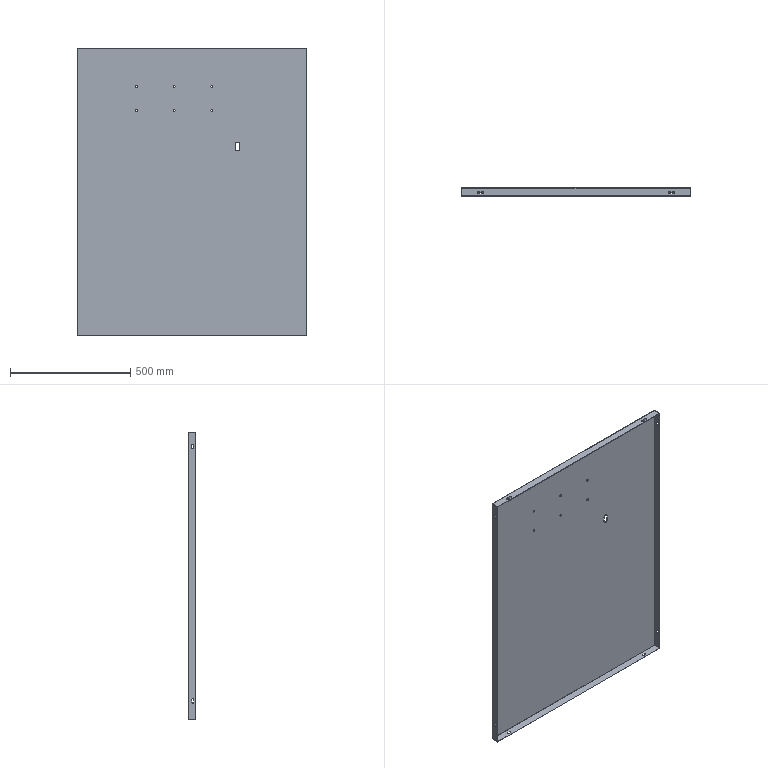Part | 1 solid | 60 faces | box 955 x 33 x 1199 mm | volume 1917439 mm3 | cylinder 31 | plane 29 | commonest cylinder face diameters 8.6 x12 9 x12 9.631 x4 17 x3